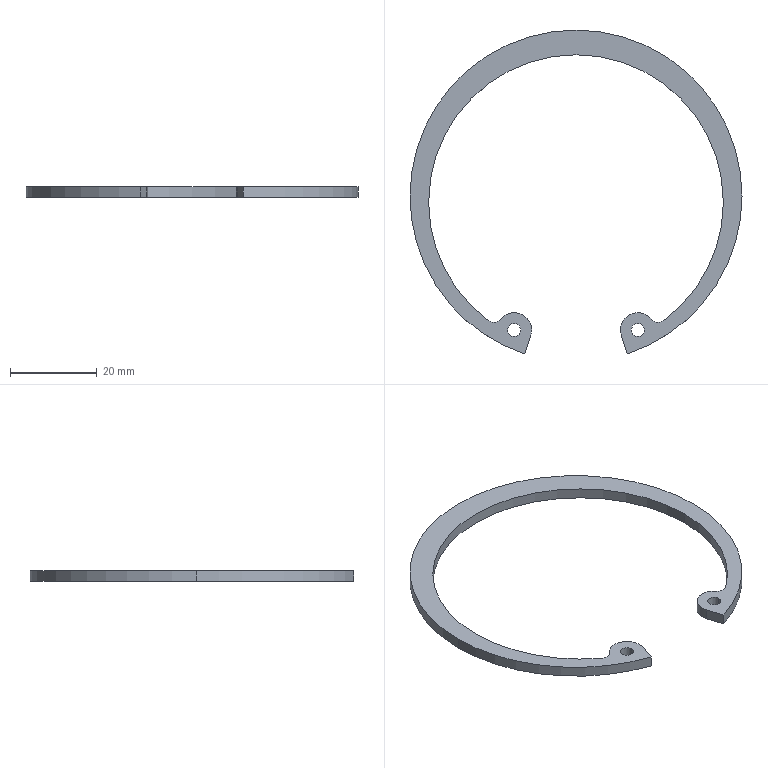Part | SolidWorks | features BaseBody 1 | 1 solid | 19 faces | box 76.5 x 74.628 x 2.5 mm | volume 2411 mm3 | cylinder 15 | plane 4 | commonest cylinder face diameters 3 x4 8 x3 67.9 x3 76.5 x3 4 x2
STEP:
#1=CARTESIAN_POINT('',(38.25,0.,-2.5));
#2=VERTEX_POINT('',#1);
#3=CARTESIAN_POINT('',(-38.25,0.,-2.5));
#4=VERTEX_POINT('',#3);
#5=CARTESIAN_POINT('',(0.,0.,-2.5));
#6=DIRECTION('',(0.,0.,1.));
#7=DIRECTION('',(1.,0.,0.));
#8=AXIS2_PLACEMENT_3D('',#5,#6,#7);
#9=CIRCLE('',#8,38.25);
#10=EDGE_CURVE('',#2,#4,#9,.T.);
#11=ORIENTED_EDGE('',*,*,#10,.T.);
#12=CARTESIAN_POINT('',(-38.25,0.,0.));
#13=VERTEX_POINT('',#12);
#14=CARTESIAN_POINT('',(-38.25,0.,-2.5));
#15=DIRECTION('',(0.,0.,1.));
#16=VECTOR('',#15,1000.);
#17=LINE('',#14,#16);
#18=EDGE_CURVE('',#4,#13,#17,.T.);
#19=ORIENTED_EDGE('',*,*,#18,.T.);
#20=CARTESIAN_POINT('',(38.25,0.,0.));
#21=VERTEX_POINT('',#20);
#22=CARTESIAN_POINT('',(0.,0.,0.));
#23=DIRECTION('',(0.,0.,-1.));
#24=DIRECTION('',(1.,0.,0.));
#25=AXIS2_PLACEMENT_3D('',#22,#23,#24);
#26=CIRCLE('',#25,38.25);
#27=EDGE_CURVE('',#13,#21,#26,.T.);
#28=ORIENTED_EDGE('',*,*,#27,.T.);
#29=CARTESIAN_POINT('',(38.25,0.,-2.5));
#30=DIRECTION('',(0.,0.,1.));
#31=VECTOR('',#30,1000.);
#32=LINE('',#29,#31);
#33=EDGE_CURVE('',#2,#21,#32,.T.);
#34=ORIENTED_EDGE('',*,*,#33,.F.);
#35=EDGE_LOOP('',(#11,#19,#28,#34));
#36=FACE_OUTER_BOUND('',#35,.T.);
#37=CARTESIAN_POINT('',(0.,0.,-2.5));
#38=DIRECTION('',(0.,0.,1.));
#39=DIRECTION('',(1.,0.,0.));
#40=AXIS2_PLACEMENT_3D('',#37,#38,#39);
#41=CYLINDRICAL_SURFACE('',#40,38.25);
#42=ADVANCED_FACE('',(#36),#41,.T.);
#43=CARTESIAN_POINT('',(11.82,-36.378,-2.5));
#44=VERTEX_POINT('',#43);
#45=CARTESIAN_POINT('',(0.,0.,-2.5));
#46=DIRECTION('',(0.,0.,1.));
#47=DIRECTION('',(1.,0.,0.));
#48=AXIS2_PLACEMENT_3D('',#45,#46,#47);
#49=CIRCLE('',#48,38.25);
#50=EDGE_CURVE('',#44,#2,#49,.T.);
#51=ORIENTED_EDGE('',*,*,#50,.T.);
#52=ORIENTED_EDGE('',*,*,#33,.T.);
#53=CARTESIAN_POINT('',(11.82,-36.378,0.));
#54=VERTEX_POINT('',#53);
#55=CARTESIAN_POINT('',(0.,0.,0.));
#56=DIRECTION('',(0.,0.,-1.));
#57=DIRECTION('',(1.,0.,0.));
#58=AXIS2_PLACEMENT_3D('',#55,#56,#57);
#59=CIRCLE('',#58,38.25);
#60=EDGE_CURVE('',#21,#54,#59,.T.);
#61=ORIENTED_EDGE('',*,*,#60,.T.);
#62=CARTESIAN_POINT('',(11.82,-36.378,-2.5));
#63=DIRECTION('',(0.,0.,-1.));
#64=VECTOR('',#63,1000.);
#65=LINE('',#62,#64);
#66=EDGE_CURVE('',#54,#44,#65,.T.);
#67=ORIENTED_EDGE('',*,*,#66,.T.);
#68=EDGE_LOOP('',(#51,#52,#61,#67));
#69=FACE_OUTER_BOUND('',#68,.T.);
#70=CARTESIAN_POINT('',(0.,0.,-2.5));
#71=DIRECTION('',(0.,0.,1.));
#72=DIRECTION('',(1.,0.,0.));
#73=AXIS2_PLACEMENT_3D('',#70,#71,#72);
#74=CYLINDRICAL_SURFACE('',#73,38.25);
#75=ADVANCED_FACE('',(#69),#74,.T.);
#76=CARTESIAN_POINT('',(-20.116,-28.748,-2.5));
#77=VERTEX_POINT('',#76);
#78=CARTESIAN_POINT('',(-33.95,-1.4,-2.5));
#79=VERTEX_POINT('',#78);
#80=CARTESIAN_POINT('',(0.,-1.4,-2.5));
#81=DIRECTION('',(0.,0.,-1.));
#82=DIRECTION('',(1.,0.,0.));
#83=AXIS2_PLACEMENT_3D('',#80,#81,#82);
#84=CIRCLE('',#83,33.95);
#85=EDGE_CURVE('',#77,#79,#84,.T.);
#86=ORIENTED_EDGE('',*,*,#85,.T.);
#87=CARTESIAN_POINT('',(-33.95,-1.4,0.));
#88=VERTEX_POINT('',#87);
#89=CARTESIAN_POINT('',(-33.95,-1.4,-2.5));
#90=DIRECTION('',(0.,0.,1.));
#91=VECTOR('',#90,1000.);
#92=LINE('',#89,#91);
#93=EDGE_CURVE('',#79,#88,#92,.T.);
#94=ORIENTED_EDGE('',*,*,#93,.T.);
#95=CARTESIAN_POINT('',(-20.116,-28.748,0.));
#96=VERTEX_POINT('',#95);
#97=CARTESIAN_POINT('',(0.,-1.4,0.));
#98=DIRECTION('',(0.,0.,-1.));
#99=DIRECTION('',(1.,0.,0.));
#100=AXIS2_PLACEMENT_3D('',#97,#98,#99);
#101=CIRCLE('',#100,33.95);
#102=EDGE_CURVE('',#96,#88,#101,.T.);
#103=ORIENTED_EDGE('',*,*,#102,.F.);
#104=CARTESIAN_POINT('',(-20.116,-28.748,-2.5));
#105=DIRECTION('',(0.,0.,1.));
#106=VECTOR('',#105,1000.);
#107=LINE('',#104,#106);
#108=EDGE_CURVE('',#77,#96,#107,.T.);
#109=ORIENTED_EDGE('',*,*,#108,.F.);
#110=EDGE_LOOP('',(#86,#94,#103,#109));
#111=FACE_OUTER_BOUND('',#110,.T.);
#112=CARTESIAN_POINT('',(0.,-1.4,-2.5));
#113=DIRECTION('',(0.,0.,1.));
#114=DIRECTION('',(1.,0.,0.));
#115=AXIS2_PLACEMENT_3D('',#112,#113,#114);
#116=CYLINDRICAL_SURFACE('',#115,33.95);
#117=ADVANCED_FACE('',(#111),#116,.F.);
#118=ORIENTED_EDGE('',*,*,#93,.F.);
#119=CARTESIAN_POINT('',(33.95,-1.4,-2.5));
#120=VERTEX_POINT('',#119);
#121=CARTESIAN_POINT('',(0.,-1.4,-2.5));
#122=DIRECTION('',(0.,0.,-1.));
#123=DIRECTION('',(1.,0.,0.));
#124=AXIS2_PLACEMENT_3D('',#121,#122,#123);
#125=CIRCLE('',#124,33.95);
#126=EDGE_CURVE('',#79,#120,#125,.T.);
#127=ORIENTED_EDGE('',*,*,#126,.T.);
#128=CARTESIAN_POINT('',(33.95,-1.4,0.));
#129=VERTEX_POINT('',#128);
#130=CARTESIAN_POINT('',(33.95,-1.4,-2.5));
#131=DIRECTION('',(0.,0.,1.));
#132=VECTOR('',#131,1000.);
#133=LINE('',#130,#132);
#134=EDGE_CURVE('',#120,#129,#133,.T.);
#135=ORIENTED_EDGE('',*,*,#134,.T.);
#136=CARTESIAN_POINT('',(0.,-1.4,0.));
#137=DIRECTION('',(0.,0.,-1.));
#138=DIRECTION('',(1.,0.,0.));
#139=AXIS2_PLACEMENT_3D('',#136,#137,#138);
#140=CIRCLE('',#139,33.95);
#141=EDGE_CURVE('',#88,#129,#140,.T.);
#142=ORIENTED_EDGE('',*,*,#141,.F.);
#143=EDGE_LOOP('',(#118,#127,#135,#142));
#144=FACE_OUTER_BOUND('',#143,.T.);
#145=CARTESIAN_POINT('',(0.,-1.4,-2.5));
#146=DIRECTION('',(0.,0.,1.));
#147=DIRECTION('',(1.,0.,0.));
#148=AXIS2_PLACEMENT_3D('',#145,#146,#147);
#149=CYLINDRICAL_SURFACE('',#148,33.95);
#150=ADVANCED_FACE('',(#144),#149,.F.);
#151=CARTESIAN_POINT('',(-10.434,-32.111,-2.5));
#152=VERTEX_POINT('',#151);
#153=CARTESIAN_POINT('',(-10.238,-30.875,-2.5));
#154=VERTEX_POINT('',#153);
#155=CARTESIAN_POINT('',(-14.238,-30.875,-2.5));
#156=DIRECTION('',(0.,0.,1.));
#157=DIRECTION('',(1.,0.,0.));
#158=AXIS2_PLACEMENT_3D('',#155,#156,#157);
#159=CIRCLE('',#158,4.);
#160=EDGE_CURVE('',#152,#154,#159,.T.);
#161=ORIENTED_EDGE('',*,*,#160,.T.);
#162=CARTESIAN_POINT('',(-10.238,-30.875,0.));
#163=VERTEX_POINT('',#162);
#164=CARTESIAN_POINT('',(-10.238,-30.875,-2.5));
#165=DIRECTION('',(0.,0.,1.));
#166=VECTOR('',#165,1000.);
#167=LINE('',#164,#166);
#168=EDGE_CURVE('',#154,#163,#167,.T.);
#169=ORIENTED_EDGE('',*,*,#168,.T.);
#170=CARTESIAN_POINT('',(-10.434,-32.111,0.));
#171=VERTEX_POINT('',#170);
#172=CARTESIAN_POINT('',(-14.238,-30.875,0.));
#173=DIRECTION('',(0.,0.,-1.));
#174=DIRECTION('',(1.,0.,0.));
#175=AXIS2_PLACEMENT_3D('',#172,#173,#174);
#176=CIRCLE('',#175,4.);
#177=EDGE_CURVE('',#163,#171,#176,.T.);
#178=ORIENTED_EDGE('',*,*,#177,.T.);
#179=CARTESIAN_POINT('',(-10.434,-32.111,-2.5));
#180=DIRECTION('',(0.,0.,1.));
#181=VECTOR('',#180,1000.);
#182=LINE('',#179,#181);
#183=EDGE_CURVE('',#152,#171,#182,.T.);
#184=ORIENTED_EDGE('',*,*,#183,.F.);
#185=EDGE_LOOP('',(#161,#169,#178,#184));
#186=FACE_OUTER_BOUND('',#185,.T.);
#187=CARTESIAN_POINT('',(-14.238,-30.875,-2.5));
#188=DIRECTION('',(0.,0.,1.));
#189=DIRECTION('',(1.,0.,0.));
#190=AXIS2_PLACEMENT_3D('',#187,#188,#189);
#191=CYLINDRICAL_SURFACE('',#190,4.);
#192=ADVANCED_FACE('',(#186),#191,.T.);
#193=CARTESIAN_POINT('',(15.738,-30.875,-2.5));
#194=VERTEX_POINT('',#193);
#195=CARTESIAN_POINT('',(12.738,-30.875,-2.5));
#196=VERTEX_POINT('',#195);
#197=CARTESIAN_POINT('',(14.238,-30.875,-2.5));
#198=DIRECTION('',(0.,0.,-1.));
#199=DIRECTION('',(1.,0.,0.));
#200=AXIS2_PLACEMENT_3D('',#197,#198,#199);
#201=CIRCLE('',#200,1.5);
#202=EDGE_CURVE('',#194,#196,#201,.T.);
#203=ORIENTED_EDGE('',*,*,#202,.T.);
#204=CARTESIAN_POINT('',(12.738,-30.875,0.));
#205=VERTEX_POINT('',#204);
#206=CARTESIAN_POINT('',(12.738,-30.875,-2.5));
#207=DIRECTION('',(0.,0.,1.));
#208=VECTOR('',#207,1000.);
#209=LINE('',#206,#208);
#210=EDGE_CURVE('',#196,#205,#209,.T.);
#211=ORIENTED_EDGE('',*,*,#210,.T.);
#212=CARTESIAN_POINT('',(15.738,-30.875,0.));
#213=VERTEX_POINT('',#212);
#214=CARTESIAN_POINT('',(14.238,-30.875,0.));
#215=DIRECTION('',(0.,0.,-1.));
#216=DIRECTION('',(1.,0.,0.));
#217=AXIS2_PLACEMENT_3D('',#214,#215,#216);
#218=CIRCLE('',#217,1.5);
#219=EDGE_CURVE('',#213,#205,#218,.T.);
#220=ORIENTED_EDGE('',*,*,#219,.F.);
#221=CARTESIAN_POINT('',(15.738,-30.875,-2.5));
#222=DIRECTION('',(0.,0.,1.));
#223=VECTOR('',#222,1000.);
#224=LINE('',#221,#223);
#225=EDGE_CURVE('',#194,#213,#224,.T.);
#226=ORIENTED_EDGE('',*,*,#225,.F.);
#227=EDGE_LOOP('',(#203,#211,#220,#226));
#228=FACE_OUTER_BOUND('',#227,.T.);
#229=CARTESIAN_POINT('',(14.238,-30.875,-2.5));
#230=DIRECTION('',(0.,0.,1.));
#231=DIRECTION('',(1.,0.,0.));
#232=AXIS2_PLACEMENT_3D('',#229,#230,#231);
#233=CYLINDRICAL_SURFACE('',#232,1.5);
#234=ADVANCED_FACE('',(#228),#233,.F.);
#235=CARTESIAN_POINT('',(-12.738,-30.875,-2.5));
#236=VERTEX_POINT('',#235);
#237=CARTESIAN_POINT('',(-15.738,-30.875,-2.5));
#238=VERTEX_POINT('',#237);
#239=CARTESIAN_POINT('',(-14.238,-30.875,-2.5));
#240=DIRECTION('',(0.,0.,-1.));
#241=DIRECTION('',(1.,0.,0.));
#242=AXIS2_PLACEMENT_3D('',#239,#240,#241);
#243=CIRCLE('',#242,1.5);
#244=EDGE_CURVE('',#236,#238,#243,.T.);
#245=ORIENTED_EDGE('',*,*,#244,.T.);
#246=CARTESIAN_POINT('',(-15.738,-30.875,0.));
#247=VERTEX_POINT('',#246);
#248=CARTESIAN_POINT('',(-15.738,-30.875,-2.5));
#249=DIRECTION('',(0.,0.,1.));
#250=VECTOR('',#249,1000.);
#251=LINE('',#248,#250);
#252=EDGE_CURVE('',#238,#247,#251,.T.);
#253=ORIENTED_EDGE('',*,*,#252,.T.);
#254=CARTESIAN_POINT('',(-12.738,-30.875,0.));
#255=VERTEX_POINT('',#254);
#256=CARTESIAN_POINT('',(-14.238,-30.875,0.));
#257=DIRECTION('',(0.,0.,-1.));
#258=DIRECTION('',(1.,0.,0.));
#259=AXIS2_PLACEMENT_3D('',#256,#257,#258);
#260=CIRCLE('',#259,1.5);
#261=EDGE_CURVE('',#255,#247,#260,.T.);
#262=ORIENTED_EDGE('',*,*,#261,.F.);
#263=CARTESIAN_POINT('',(-12.738,-30.875,-2.5));
#264=DIRECTION('',(0.,0.,1.));
#265=VECTOR('',#264,1000.);
#266=LINE('',#263,#265);
#267=EDGE_CURVE('',#236,#255,#266,.T.);
#268=ORIENTED_EDGE('',*,*,#267,.F.);
#269=EDGE_LOOP('',(#245,#253,#262,#268));
#270=FACE_OUTER_BOUND('',#269,.T.);
#271=CARTESIAN_POINT('',(-14.238,-30.875,-2.5));
#272=DIRECTION('',(0.,0.,1.));
#273=DIRECTION('',(1.,0.,0.));
#274=AXIS2_PLACEMENT_3D('',#271,#272,#273);
#275=CYLINDRICAL_SURFACE('',#274,1.5);
#276=ADVANCED_FACE('',(#270),#275,.F.);
#277=CARTESIAN_POINT('',(10.434,-32.111,-2.5));
#278=VERTEX_POINT('',#277);
#279=CARTESIAN_POINT('',(10.434,-32.111,-2.5));
#280=DIRECTION('',(0.309,-0.9511,0.));
#281=VECTOR('',#280,1000.);
#282=LINE('',#279,#281);
#283=EDGE_CURVE('',#278,#44,#282,.T.);
#284=ORIENTED_EDGE('',*,*,#283,.F.);
#285=CARTESIAN_POINT('',(17.367,-28.383,-2.5));
#286=VERTEX_POINT('',#285);
#287=CARTESIAN_POINT('',(14.238,-30.875,-2.5));
#288=DIRECTION('',(0.,0.,1.));
#289=DIRECTION('',(1.,0.,0.));
#290=AXIS2_PLACEMENT_3D('',#287,#288,#289);
#291=CIRCLE('',#290,4.);
#292=EDGE_CURVE('',#286,#278,#291,.T.);
#293=ORIENTED_EDGE('',*,*,#292,.F.);
#294=CARTESIAN_POINT('',(20.116,-28.748,-2.5));
#295=VERTEX_POINT('',#294);
#296=CARTESIAN_POINT('',(18.931,-27.137,-2.5));
#297=DIRECTION('',(0.,0.,-1.));
#298=DIRECTION('',(1.,0.,0.));
#299=AXIS2_PLACEMENT_3D('',#296,#297,#298);
#300=CIRCLE('',#299,2.);
#301=EDGE_CURVE('',#295,#286,#300,.T.);
#302=ORIENTED_EDGE('',*,*,#301,.F.);
#303=CARTESIAN_POINT('',(0.,-1.4,-2.5));
#304=DIRECTION('',(0.,0.,-1.));
#305=DIRECTION('',(1.,0.,0.));
#306=AXIS2_PLACEMENT_3D('',#303,#304,#305);
#307=CIRCLE('',#306,33.95);
#308=EDGE_CURVE('',#120,#295,#307,.T.);
#309=ORIENTED_EDGE('',*,*,#308,.F.);
#310=ORIENTED_EDGE('',*,*,#126,.F.);
#311=ORIENTED_EDGE('',*,*,#85,.F.);
#312=CARTESIAN_POINT('',(-17.367,-28.383,-2.5));
#313=VERTEX_POINT('',#312);
#314=CARTESIAN_POINT('',(-18.931,-27.137,-2.5));
#315=DIRECTION('',(0.,0.,-1.));
#316=DIRECTION('',(1.,0.,0.));
#317=AXIS2_PLACEMENT_3D('',#314,#315,#316);
#318=CIRCLE('',#317,2.);
#319=EDGE_CURVE('',#313,#77,#318,.T.);
#320=ORIENTED_EDGE('',*,*,#319,.F.);
#321=CARTESIAN_POINT('',(-14.238,-30.875,-2.5));
#322=DIRECTION('',(0.,0.,1.));
#323=DIRECTION('',(1.,0.,0.));
#324=AXIS2_PLACEMENT_3D('',#321,#322,#323);
#325=CIRCLE('',#324,4.);
#326=EDGE_CURVE('',#154,#313,#325,.T.);
#327=ORIENTED_EDGE('',*,*,#326,.F.);
#328=ORIENTED_EDGE('',*,*,#160,.F.);
#329=CARTESIAN_POINT('',(-11.82,-36.378,-2.5));
#330=VERTEX_POINT('',#329);
#331=CARTESIAN_POINT('',(-11.82,-36.378,-2.5));
#332=DIRECTION('',(0.309,0.9511,0.));
#333=VECTOR('',#332,1000.);
#334=LINE('',#331,#333);
#335=EDGE_CURVE('',#330,#152,#334,.T.);
#336=ORIENTED_EDGE('',*,*,#335,.F.);
#337=CARTESIAN_POINT('',(0.,0.,-2.5));
#338=DIRECTION('',(0.,0.,1.));
#339=DIRECTION('',(1.,0.,0.));
#340=AXIS2_PLACEMENT_3D('',#337,#338,#339);
#341=CIRCLE('',#340,38.25);
#342=EDGE_CURVE('',#4,#330,#341,.T.);
#343=ORIENTED_EDGE('',*,*,#342,.F.);
#344=ORIENTED_EDGE('',*,*,#10,.F.);
#345=ORIENTED_EDGE('',*,*,#50,.F.);
#346=EDGE_LOOP('',(#284,#293,#302,#309,#310,#311,#320,#327,#328,#336,#343,#344,#345));
#347=FACE_OUTER_BOUND('',#346,.T.);
#348=ORIENTED_EDGE('',*,*,#202,.F.);
#349=CARTESIAN_POINT('',(14.238,-30.875,-2.5));
#350=DIRECTION('',(0.,0.,-1.));
#351=DIRECTION('',(1.,0.,0.));
#352=AXIS2_PLACEMENT_3D('',#349,#350,#351);
#353=CIRCLE('',#352,1.5);
#354=EDGE_CURVE('',#196,#194,#353,.T.);
#355=ORIENTED_EDGE('',*,*,#354,.F.);
#356=EDGE_LOOP('',(#348,#355));
#357=FACE_BOUND('',#356,.T.);
#358=ORIENTED_EDGE('',*,*,#244,.F.);
#359=CARTESIAN_POINT('',(-14.238,-30.875,-2.5));
#360=DIRECTION('',(0.,0.,-1.));
#361=DIRECTION('',(1.,0.,0.));
#362=AXIS2_PLACEMENT_3D('',#359,#360,#361);
#363=CIRCLE('',#362,1.5);
#364=EDGE_CURVE('',#238,#236,#363,.T.);
#365=ORIENTED_EDGE('',*,*,#364,.F.);
#366=EDGE_LOOP('',(#358,#365));
#367=FACE_BOUND('',#366,.T.);
#368=CARTESIAN_POINT('',(0.,0.,-2.5));
#369=DIRECTION('',(0.,0.,1.));
#370=DIRECTION('',(1.,0.,0.));
#371=AXIS2_PLACEMENT_3D('',#368,#369,#370);
#372=PLANE('',#371);
#373=ADVANCED_FACE('',(#347,#357,#367),#372,.F.);
#374=ORIENTED_EDGE('',*,*,#18,.F.);
#375=ORIENTED_EDGE('',*,*,#342,.T.);
#376=CARTESIAN_POINT('',(-11.82,-36.378,0.));
#377=VERTEX_POINT('',#376);
#378=CARTESIAN_POINT('',(-11.82,-36.378,-2.5));
#379=DIRECTION('',(0.,0.,-1.));
#380=VECTOR('',#379,1000.);
#381=LINE('',#378,#380);
#382=EDGE_CURVE('',#377,#330,#381,.T.);
#383=ORIENTED_EDGE('',*,*,#382,.F.);
#384=CARTESIAN_POINT('',(0.,0.,0.));
#385=DIRECTION('',(0.,0.,-1.));
#386=DIRECTION('',(1.,0.,0.));
#387=AXIS2_PLACEMENT_3D('',#384,#385,#386);
#388=CIRCLE('',#387,38.25);
#389=EDGE_CURVE('',#377,#13,#388,.T.);
#390=ORIENTED_EDGE('',*,*,#389,.T.);
#391=EDGE_LOOP('',(#374,#375,#383,#390));
#392=FACE_OUTER_BOUND('',#391,.T.);
#393=CARTESIAN_POINT('',(0.,0.,-2.5));
#394=DIRECTION('',(0.,0.,1.));
#395=DIRECTION('',(1.,0.,0.));
#396=AXIS2_PLACEMENT_3D('',#393,#394,#395);
#397=CYLINDRICAL_SURFACE('',#396,38.25);
#398=ADVANCED_FACE('',(#392),#397,.T.);
#399=ORIENTED_EDGE('',*,*,#283,.T.);
#400=ORIENTED_EDGE('',*,*,#66,.F.);
#401=CARTESIAN_POINT('',(10.434,-32.111,0.));
#402=VERTEX_POINT('',#401);
#403=CARTESIAN_POINT('',(10.434,-32.111,0.));
#404=DIRECTION('',(-0.309,0.9511,0.));
#405=VECTOR('',#404,1000.);
#406=LINE('',#403,#405);
#407=EDGE_CURVE('',#54,#402,#406,.T.);
#408=ORIENTED_EDGE('',*,*,#407,.T.);
#409=CARTESIAN_POINT('',(10.434,-32.111,-2.5));
#410=DIRECTION('',(0.,0.,-1.));
#411=VECTOR('',#410,1000.);
#412=LINE('',#409,#411);
#413=EDGE_CURVE('',#402,#278,#412,.T.);
#414=ORIENTED_EDGE('',*,*,#413,.T.);
#415=EDGE_LOOP('',(#399,#400,#408,#414));
#416=FACE_OUTER_BOUND('',#415,.T.);
#417=CARTESIAN_POINT('',(10.434,-32.111,-2.5));
#418=DIRECTION('',(-0.9511,-0.309,0.));
#419=DIRECTION('',(0.309,-0.9511,0.));
#420=AXIS2_PLACEMENT_3D('',#417,#418,#419);
#421=PLANE('',#420);
#422=ADVANCED_FACE('',(#416),#421,.T.);
#423=ORIENTED_EDGE('',*,*,#292,.T.);
#424=ORIENTED_EDGE('',*,*,#413,.F.);
#425=CARTESIAN_POINT('',(17.367,-28.383,0.));
#426=VERTEX_POINT('',#425);
#427=CARTESIAN_POINT('',(14.238,-30.875,0.));
#428=DIRECTION('',(0.,0.,-1.));
#429=DIRECTION('',(1.,0.,0.));
#430=AXIS2_PLACEMENT_3D('',#427,#428,#429);
#431=CIRCLE('',#430,4.);
#432=EDGE_CURVE('',#402,#426,#431,.T.);
#433=ORIENTED_EDGE('',*,*,#432,.T.);
#434=CARTESIAN_POINT('',(17.367,-28.383,-2.5));
#435=DIRECTION('',(0.,0.,-1.));
#436=VECTOR('',#435,1000.);
#437=LINE('',#434,#436);
#438=EDGE_CURVE('',#426,#286,#437,.T.);
#439=ORIENTED_EDGE('',*,*,#438,.T.);
#440=EDGE_LOOP('',(#423,#424,#433,#439));
#441=FACE_OUTER_BOUND('',#440,.T.);
#442=CARTESIAN_POINT('',(14.238,-30.875,-2.5));
#443=DIRECTION('',(0.,0.,1.));
#444=DIRECTION('',(1.,0.,0.));
#445=AXIS2_PLACEMENT_3D('',#442,#443,#444);
#446=CYLINDRICAL_SURFACE('',#445,4.);
#447=ADVANCED_FACE('',(#441),#446,.T.);
#448=CARTESIAN_POINT('',(20.116,-28.748,0.));
#449=VERTEX_POINT('',#448);
#450=CARTESIAN_POINT('',(20.116,-28.748,-2.5));
#451=DIRECTION('',(0.,0.,1.));
#452=VECTOR('',#451,1000.);
#453=LINE('',#450,#452);
#454=EDGE_CURVE('',#295,#449,#453,.T.);
#455=ORIENTED_EDGE('',*,*,#454,.F.);
#456=ORIENTED_EDGE('',*,*,#301,.T.);
#457=ORIENTED_EDGE('',*,*,#438,.F.);
#458=CARTESIAN_POINT('',(18.931,-27.137,0.));
#459=DIRECTION('',(0.,0.,-1.));
#460=DIRECTION('',(1.,0.,0.));
#461=AXIS2_PLACEMENT_3D('',#458,#459,#460);
#462=CIRCLE('',#461,2.);
#463=EDGE_CURVE('',#449,#426,#462,.T.);
#464=ORIENTED_EDGE('',*,*,#463,.F.);
#465=EDGE_LOOP('',(#455,#456,#457,#464));
#466=FACE_OUTER_BOUND('',#465,.T.);
#467=CARTESIAN_POINT('',(18.931,-27.137,-2.5));
#468=DIRECTION('',(0.,0.,1.));
#469=DIRECTION('',(1.,0.,0.));
#470=AXIS2_PLACEMENT_3D('',#467,#468,#469);
#471=CYLINDRICAL_SURFACE('',#470,2.);
#472=ADVANCED_FACE('',(#466),#471,.F.);
#473=ORIENTED_EDGE('',*,*,#134,.F.);
#474=ORIENTED_EDGE('',*,*,#308,.T.);
#475=ORIENTED_EDGE('',*,*,#454,.T.);
#476=CARTESIAN_POINT('',(0.,-1.4,0.));
#477=DIRECTION('',(0.,0.,-1.));
#478=DIRECTION('',(1.,0.,0.));
#479=AXIS2_PLACEMENT_3D('',#476,#477,#478);
#480=CIRCLE('',#479,33.95);
#481=EDGE_CURVE('',#129,#449,#480,.T.);
#482=ORIENTED_EDGE('',*,*,#481,.F.);
#483=EDGE_LOOP('',(#473,#474,#475,#482));
#484=FACE_OUTER_BOUND('',#483,.T.);
#485=CARTESIAN_POINT('',(0.,-1.4,-2.5));
#486=DIRECTION('',(0.,0.,1.));
#487=DIRECTION('',(1.,0.,0.));
#488=AXIS2_PLACEMENT_3D('',#485,#486,#487);
#489=CYLINDRICAL_SURFACE('',#488,33.95);
#490=ADVANCED_FACE('',(#484),#489,.F.);
#491=CARTESIAN_POINT('',(-17.367,-28.383,0.));
#492=VERTEX_POINT('',#491);
#493=CARTESIAN_POINT('',(-17.367,-28.383,-2.5));
#494=DIRECTION('',(0.,0.,1.));
#495=VECTOR('',#494,1000.);
#496=LINE('',#493,#495);
#497=EDGE_CURVE('',#313,#492,#496,.T.);
#498=ORIENTED_EDGE('',*,*,#497,.F.);
#499=ORIENTED_EDGE('',*,*,#319,.T.);
#500=ORIENTED_EDGE('',*,*,#108,.T.);
#501=CARTESIAN_POINT('',(-18.931,-27.137,0.));
#502=DIRECTION('',(0.,0.,-1.));
#503=DIRECTION('',(1.,0.,0.));
#504=AXIS2_PLACEMENT_3D('',#501,#502,#503);
#505=CIRCLE('',#504,2.);
#506=EDGE_CURVE('',#492,#96,#505,.T.);
#507=ORIENTED_EDGE('',*,*,#506,.F.);
#508=EDGE_LOOP('',(#498,#499,#500,#507));
#509=FACE_OUTER_BOUND('',#508,.T.);
#510=CARTESIAN_POINT('',(-18.931,-27.137,-2.5));
#511=DIRECTION('',(0.,0.,1.));
#512=DIRECTION('',(1.,0.,0.));
#513=AXIS2_PLACEMENT_3D('',#510,#511,#512);
#514=CYLINDRICAL_SURFACE('',#513,2.);
#515=ADVANCED_FACE('',(#509),#514,.F.);
#516=ORIENTED_EDGE('',*,*,#168,.F.);
#517=ORIENTED_EDGE('',*,*,#326,.T.);
#518=ORIENTED_EDGE('',*,*,#497,.T.);
#519=CARTESIAN_POINT('',(-14.238,-30.875,0.));
#520=DIRECTION('',(0.,0.,-1.));
#521=DIRECTION('',(1.,0.,0.));
#522=AXIS2_PLACEMENT_3D('',#519,#520,#521);
#523=CIRCLE('',#522,4.);
#524=EDGE_CURVE('',#492,#163,#523,.T.);
#525=ORIENTED_EDGE('',*,*,#524,.T.);
#526=EDGE_LOOP('',(#516,#517,#518,#525));
#527=FACE_OUTER_BOUND('',#526,.T.);
#528=CARTESIAN_POINT('',(-14.238,-30.875,-2.5));
#529=DIRECTION('',(0.,0.,1.));
#530=DIRECTION('',(1.,0.,0.));
#531=AXIS2_PLACEMENT_3D('',#528,#529,#530);
#532=CYLINDRICAL_SURFACE('',#531,4.);
#533=ADVANCED_FACE('',(#527),#532,.T.);
#534=ORIENTED_EDGE('',*,*,#335,.T.);
#535=ORIENTED_EDGE('',*,*,#183,.T.);
#536=CARTESIAN_POINT('',(-10.434,-32.111,0.));
#537=DIRECTION('',(-0.309,-0.9511,0.));
#538=VECTOR('',#537,1000.);
#539=LINE('',#536,#538);
#540=EDGE_CURVE('',#171,#377,#539,.T.);
#541=ORIENTED_EDGE('',*,*,#540,.T.);
#542=ORIENTED_EDGE('',*,*,#382,.T.);
#543=EDGE_LOOP('',(#534,#535,#541,#542));
#544=FACE_OUTER_BOUND('',#543,.T.);
#545=CARTESIAN_POINT('',(-10.434,-32.111,-2.5));
#546=DIRECTION('',(0.9511,-0.309,0.));
#547=DIRECTION('',(0.309,0.9511,0.));
#548=AXIS2_PLACEMENT_3D('',#545,#546,#547);
#549=PLANE('',#548);
#550=ADVANCED_FACE('',(#544),#549,.T.);
#551=ORIENTED_EDGE('',*,*,#210,.F.);
#552=ORIENTED_EDGE('',*,*,#354,.T.);
#553=ORIENTED_EDGE('',*,*,#225,.T.);
#554=CARTESIAN_POINT('',(14.238,-30.875,0.));
#555=DIRECTION('',(0.,0.,-1.));
#556=DIRECTION('',(1.,0.,0.));
#557=AXIS2_PLACEMENT_3D('',#554,#555,#556);
#558=CIRCLE('',#557,1.5);
#559=EDGE_CURVE('',#205,#213,#558,.T.);
#560=ORIENTED_EDGE('',*,*,#559,.F.);
#561=EDGE_LOOP('',(#551,#552,#553,#560));
#562=FACE_OUTER_BOUND('',#561,.T.);
#563=CARTESIAN_POINT('',(14.238,-30.875,-2.5));
#564=DIRECTION('',(0.,0.,1.));
#565=DIRECTION('',(1.,0.,0.));
#566=AXIS2_PLACEMENT_3D('',#563,#564,#565);
#567=CYLINDRICAL_SURFACE('',#566,1.5);
#568=ADVANCED_FACE('',(#562),#567,.F.);
#569=ORIENTED_EDGE('',*,*,#252,.F.);
#570=ORIENTED_EDGE('',*,*,#364,.T.);
#571=ORIENTED_EDGE('',*,*,#267,.T.);
#572=CARTESIAN_POINT('',(-14.238,-30.875,0.));
#573=DIRECTION('',(0.,0.,-1.));
#574=DIRECTION('',(1.,0.,0.));
#575=AXIS2_PLACEMENT_3D('',#572,#573,#574);
#576=CIRCLE('',#575,1.5);
#577=EDGE_CURVE('',#247,#255,#576,.T.);
#578=ORIENTED_EDGE('',*,*,#577,.F.);
#579=EDGE_LOOP('',(#569,#570,#571,#578));
#580=FACE_OUTER_BOUND('',#579,.T.);
#581=CARTESIAN_POINT('',(-14.238,-30.875,-2.5));
#582=DIRECTION('',(0.,0.,1.));
#583=DIRECTION('',(1.,0.,0.));
#584=AXIS2_PLACEMENT_3D('',#581,#582,#583);
#585=CYLINDRICAL_SURFACE('',#584,1.5);
#586=ADVANCED_FACE('',(#580),#585,.F.);
#587=ORIENTED_EDGE('',*,*,#432,.F.);
#588=ORIENTED_EDGE('',*,*,#407,.F.);
#589=ORIENTED_EDGE('',*,*,#60,.F.);
#590=ORIENTED_EDGE('',*,*,#27,.F.);
#591=ORIENTED_EDGE('',*,*,#389,.F.);
#592=ORIENTED_EDGE('',*,*,#540,.F.);
#593=ORIENTED_EDGE('',*,*,#177,.F.);
#594=ORIENTED_EDGE('',*,*,#524,.F.);
#595=ORIENTED_EDGE('',*,*,#506,.T.);
#596=ORIENTED_EDGE('',*,*,#102,.T.);
#597=ORIENTED_EDGE('',*,*,#141,.T.);
#598=ORIENTED_EDGE('',*,*,#481,.T.);
#599=ORIENTED_EDGE('',*,*,#463,.T.);
#600=EDGE_LOOP('',(#587,#588,#589,#590,#591,#592,#593,#594,#595,#596,#597,#598,#599));
#601=FACE_OUTER_BOUND('',#600,.T.);
#602=ORIENTED_EDGE('',*,*,#219,.T.);
#603=ORIENTED_EDGE('',*,*,#559,.T.);
#604=EDGE_LOOP('',(#602,#603));
#605=FACE_BOUND('',#604,.T.);
#606=ORIENTED_EDGE('',*,*,#261,.T.);
#607=ORIENTED_EDGE('',*,*,#577,.T.);
#608=EDGE_LOOP('',(#606,#607));
#609=FACE_BOUND('',#608,.T.);
#610=CARTESIAN_POINT('',(0.,0.,0.));
#611=DIRECTION('',(0.,0.,1.));
#612=DIRECTION('',(1.,0.,0.));
#613=AXIS2_PLACEMENT_3D('',#610,#611,#612);
#614=PLANE('',#613);
#615=ADVANCED_FACE('',(#601,#605,#609),#614,.T.);
#616=CLOSED_SHELL('',(#42,#75,#117,#150,#192,#234,#276,#373,#398,#422,#447,#472,#490,#515,#533,#550,#568,#586,#615));
#617=MANIFOLD_SOLID_BREP('',#616);
#618=CARTESIAN_POINT('',(0.,0.,0.));
#619=DIRECTION('',(0.,0.,1.));
#620=DIRECTION('',(1.,0.,0.));
#621=AXIS2_PLACEMENT_3D('',#618,#619,#620);
#622=(LENGTH_UNIT()NAMED_UNIT(*)SI_UNIT(.MILLI.,.METRE.));
#623=UNCERTAINTY_MEASURE_WITH_UNIT(LENGTH_MEASURE(0.00001),#622,'','');
#624=(NAMED_UNIT(*)PLANE_ANGLE_UNIT()SI_UNIT($,.RADIAN.));
#625=(NAMED_UNIT(*)SI_UNIT($,.STERADIAN.)SOLID_ANGLE_UNIT());
#626=(GEOMETRIC_REPRESENTATION_CONTEXT(3)GLOBAL_UNCERTAINTY_ASSIGNED_CONTEXT((#623))GLOBAL_UNIT_ASSIGNED_CONTEXT((#622,#624,#625))REPRESENTATION_CONTEXT('',''));
#627=ADVANCED_BREP_SHAPE_REPRESENTATION('',(#617,#621),#626);